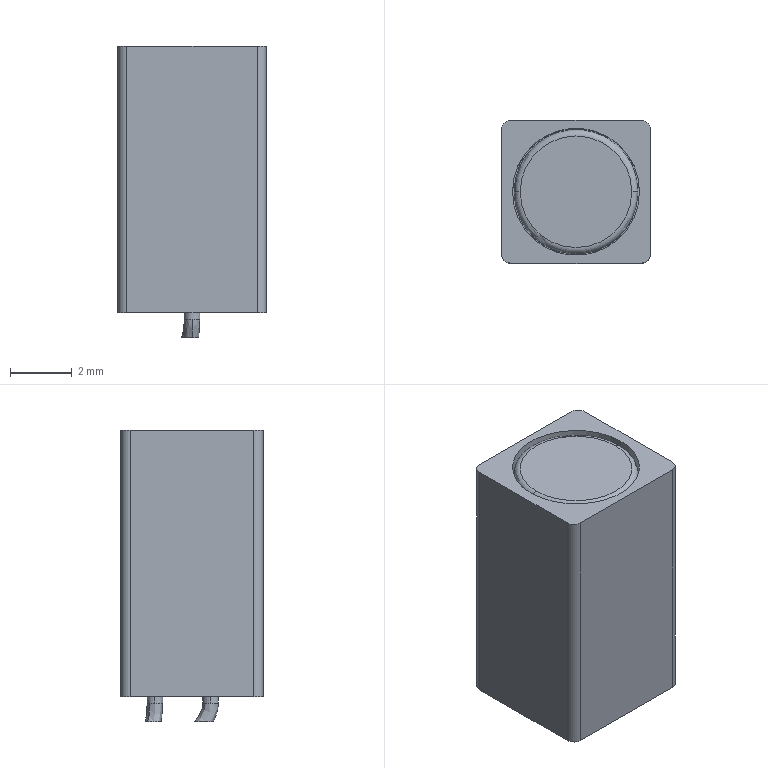Part | Creo | 1 solid | 33 faces | box 4.8 x 4.6 x 9.4 mm | volume 182.133 mm3 | cylinder 14 | plane 13 | spline 4 | torus 2 | commonest cylinder face diameters 0.5 x4 0.6 x4 0.98 x2 4 x2 4.1 x2
STEP:
#1=CARTESIAN_POINT('',(0.,0.,0.));
#2=DIRECTION('',(0.,0.,1.));
#3=DIRECTION('',(1.,0.,0.));
#4=AXIS2_PLACEMENT_3D('',#1,#2,#3);
#5=CARTESIAN_POINT('',(2.498,1.613,-0.6));
#6=VERTEX_POINT('',#5);
#7=CARTESIAN_POINT('',(2.417,2.21,-0.6));
#8=VERTEX_POINT('',#7);
#9=CARTESIAN_POINT('',(2.508,1.614,-0.6));
#10=CARTESIAN_POINT('',(2.527,1.617,-0.6));
#11=CARTESIAN_POINT('',(2.557,1.626,-0.6));
#12=CARTESIAN_POINT('',(2.585,1.64,-0.6));
#13=CARTESIAN_POINT('',(2.612,1.657,-0.6));
#14=CARTESIAN_POINT('',(2.636,1.678,-0.6));
#15=CARTESIAN_POINT('',(2.658,1.703,-0.6));
#16=CARTESIAN_POINT('',(2.676,1.73,-0.6));
#17=CARTESIAN_POINT('',(2.692,1.762,-0.6));
#18=CARTESIAN_POINT('',(2.704,1.798,-0.6));
#19=CARTESIAN_POINT('',(2.712,1.836,-0.6));
#20=CARTESIAN_POINT('',(2.715,1.877,-0.6));
#21=CARTESIAN_POINT('',(2.713,1.918,-0.6));
#22=CARTESIAN_POINT('',(2.706,1.959,-0.6));
#23=CARTESIAN_POINT('',(2.693,2.001,-0.6));
#24=CARTESIAN_POINT('',(2.675,2.043,-0.6));
#25=CARTESIAN_POINT('',(2.652,2.08,-0.6));
#26=CARTESIAN_POINT('',(2.626,2.114,-0.6));
#27=CARTESIAN_POINT('',(2.598,2.142,-0.6));
#28=CARTESIAN_POINT('',(2.568,2.166,-0.6));
#29=CARTESIAN_POINT('',(2.537,2.184,-0.6));
#30=CARTESIAN_POINT('',(2.505,2.198,-0.6));
#31=CARTESIAN_POINT('',(2.474,2.207,-0.6));
#32=CARTESIAN_POINT('',(2.444,2.211,-0.6));
#33=CARTESIAN_POINT('',(2.426,2.211,-0.6));
#34=B_SPLINE_CURVE_WITH_KNOTS('',3,(#5,#9,#10,#11,#12,#13,#14,#15,#16,#17,#18,#19,#20,#21,#22,#23,#24,#25,#26,#27,#28,#29,#30,#31,#32,#33,#7),.UNSPECIFIED.,.F.,.F.,(4,1,1,1,1,1,1,1,1,1,1,1,1,1,1,1,1,1,1,1,1,1,1,1,4),(0.,0.04167,0.08333,0.125,0.1667,0.2083,0.25,0.2917,0.3333,0.375,0.4167,0.4583,0.5,0.5417,0.5833,0.625,0.6667,0.7083,0.75,0.7917,0.8333,0.875,0.9167,0.9583,1.),.UNSPECIFIED.);
#35=EDGE_CURVE('',#6,#8,#34,.T.);
#36=ORIENTED_EDGE('',*,*,#35,.F.);
#37=CARTESIAN_POINT('',(2.526,1.451,0.));
#38=VERTEX_POINT('',#37);
#39=CARTESIAN_POINT('',(2.498,1.613,-0.6));
#40=CARTESIAN_POINT('',(2.506,1.577,-0.5309));
#41=CARTESIAN_POINT('',(2.521,1.494,-0.3468));
#42=CARTESIAN_POINT('',(2.526,1.451,-0.1342));
#43=B_SPLINE_CURVE_WITH_KNOTS('',3,(#39,#40,#41,#42,#37),.UNSPECIFIED.,.F.,.F.,(4,1,4),(0.,0.3969,1.),.UNSPECIFIED.);
#44=EDGE_CURVE('',#6,#38,#43,.T.);
#45=ORIENTED_EDGE('',*,*,#44,.T.);
#46=CARTESIAN_POINT('',(2.75,1.7,0.));
#47=VERTEX_POINT('',#46);
#48=CARTESIAN_POINT('',(2.5,1.7,0.));
#49=DIRECTION('',(0.,0.,1.));
#50=DIRECTION('',(0.1037,-0.9946,0.));
#51=AXIS2_PLACEMENT_3D('',#48,#49,#50);
#52=CIRCLE('',#51,0.25);
#53=EDGE_CURVE('',#38,#47,#52,.T.);
#54=ORIENTED_EDGE('',*,*,#53,.T.);
#55=CARTESIAN_POINT('',(2.474,1.949,0.));
#56=VERTEX_POINT('',#55);
#57=CARTESIAN_POINT('',(2.5,1.7,0.));
#58=DIRECTION('',(0.,0.,1.));
#59=DIRECTION('',(1.,0.000000353,0.));
#60=AXIS2_PLACEMENT_3D('',#57,#58,#59);
#61=CIRCLE('',#60,0.25);
#62=EDGE_CURVE('',#47,#56,#61,.T.);
#63=ORIENTED_EDGE('',*,*,#62,.T.);
#64=CARTESIAN_POINT('',(2.417,2.21,-0.6));
#65=CARTESIAN_POINT('',(2.427,2.173,-0.5544));
#66=CARTESIAN_POINT('',(2.451,2.083,-0.4299));
#67=CARTESIAN_POINT('',(2.471,1.978,-0.2252));
#68=CARTESIAN_POINT('',(2.474,1.949,-0.06818));
#69=CARTESIAN_POINT('',(2.474,1.949,0.));
#70=B_SPLINE_CURVE_WITH_KNOTS('',3,(#64,#65,#66,#67,#68,#69),.UNSPECIFIED.,.F.,.F.,(4,1,1,4),(0.,0.24,0.6382,1.),.UNSPECIFIED.);
#71=EDGE_CURVE('',#8,#56,#70,.T.);
#72=ORIENTED_EDGE('',*,*,#71,.F.);
#73=EDGE_LOOP('',(#36,#45,#54,#63,#72));
#74=FACE_OUTER_BOUND('',#73,.F.);
#75=CARTESIAN_POINT('',(2.466,1.948,0.006392));
#76=CARTESIAN_POINT('',(2.466,1.947,-0.06352));
#77=CARTESIAN_POINT('',(2.464,1.976,-0.2228));
#78=CARTESIAN_POINT('',(2.443,2.083,-0.4318));
#79=CARTESIAN_POINT('',(2.419,2.175,-0.5581));
#80=CARTESIAN_POINT('',(2.407,2.214,-0.6057));
#81=CARTESIAN_POINT('',(2.469,1.948,0.006391));
#82=CARTESIAN_POINT('',(2.469,1.947,-0.06351));
#83=CARTESIAN_POINT('',(2.466,1.976,-0.2228));
#84=CARTESIAN_POINT('',(2.446,2.083,-0.4319));
#85=CARTESIAN_POINT('',(2.421,2.176,-0.5583));
#86=CARTESIAN_POINT('',(2.41,2.214,-0.6059));
#87=CARTESIAN_POINT('',(2.536,1.956,0.006376));
#88=CARTESIAN_POINT('',(2.536,1.955,-0.06333));
#89=CARTESIAN_POINT('',(2.534,1.984,-0.2235));
#90=CARTESIAN_POINT('',(2.513,2.093,-0.4355));
#91=CARTESIAN_POINT('',(2.488,2.187,-0.5639));
#92=CARTESIAN_POINT('',(2.477,2.226,-0.6123));
#93=CARTESIAN_POINT('',(2.675,1.915,0.007061));
#94=CARTESIAN_POINT('',(2.675,1.914,-0.07018));
#95=CARTESIAN_POINT('',(2.672,1.946,-0.2451));
#96=CARTESIAN_POINT('',(2.649,2.063,-0.4733));
#97=CARTESIAN_POINT('',(2.623,2.163,-0.6099));
#98=CARTESIAN_POINT('',(2.611,2.204,-0.6613));
#99=CARTESIAN_POINT('',(2.776,1.729,0.009505));
#100=CARTESIAN_POINT('',(2.776,1.727,-0.09468));
#101=CARTESIAN_POINT('',(2.772,1.769,-0.3159));
#102=CARTESIAN_POINT('',(2.745,1.908,-0.5835));
#103=CARTESIAN_POINT('',(2.715,2.02,-0.7374));
#104=CARTESIAN_POINT('',(2.701,2.067,-0.7945));
#105=CARTESIAN_POINT('',(2.715,1.526,0.01195));
#106=CARTESIAN_POINT('',(2.715,1.524,-0.1193));
#107=CARTESIAN_POINT('',(2.71,1.576,-0.3841));
#108=CARTESIAN_POINT('',(2.68,1.732,-0.6839));
#109=CARTESIAN_POINT('',(2.647,1.854,-0.8498));
#110=CARTESIAN_POINT('',(2.633,1.903,-0.9108));
#111=CARTESIAN_POINT('',(2.588,1.457,0.01264));
#112=CARTESIAN_POINT('',(2.589,1.455,-0.1262));
#113=CARTESIAN_POINT('',(2.583,1.51,-0.4016));
#114=CARTESIAN_POINT('',(2.552,1.669,-0.7055));
#115=CARTESIAN_POINT('',(2.519,1.79,-0.8713));
#116=CARTESIAN_POINT('',(2.505,1.84,-0.9321));
#117=CARTESIAN_POINT('',(2.521,1.451,0.01263));
#118=CARTESIAN_POINT('',(2.521,1.449,-0.1261));
#119=CARTESIAN_POINT('',(2.515,1.504,-0.4002));
#120=CARTESIAN_POINT('',(2.485,1.661,-0.7008));
#121=CARTESIAN_POINT('',(2.453,1.781,-0.8644));
#122=CARTESIAN_POINT('',(2.438,1.83,-0.9243));
#123=CARTESIAN_POINT('',(2.518,1.451,0.01263));
#124=CARTESIAN_POINT('',(2.518,1.449,-0.1261));
#125=CARTESIAN_POINT('',(2.513,1.504,-0.4001));
#126=CARTESIAN_POINT('',(2.482,1.661,-0.7006));
#127=CARTESIAN_POINT('',(2.45,1.781,-0.8641));
#128=CARTESIAN_POINT('',(2.436,1.829,-0.924));
#129=B_SPLINE_SURFACE_WITH_KNOTS('',3,3,((#75,#76,#77,#78,#79,#80),(#81,#82,#83,#84,#85,#86),(#87,#88,#89,#90,#91,#92),(#93,#94,#95,#96,#97,#98),(#99,#100,#101,#102,#103,#104),(#105,#106,#107,#108,#109,#110),(#111,#112,#113,#114,#115,#116),(#117,#118,#119,#120,#121,#122),(#123,#124,#125,#126,#127,#128)),.UNSPECIFIED.,.F.,.F.,.F.,(4,1,1,1,1,1,4),(4,1,1,4),(-0.004999,0.,0.125,0.25,0.375,0.5,0.505),(-0.009526,0.304,0.6386,0.8497),.UNSPECIFIED.);
#130=ADVANCED_FACE('',(#74),#129,.T.);
#131=ORIENTED_EDGE('',*,*,#35,.T.);
#132=CARTESIAN_POINT('',(2.417,2.21,-0.6));
#133=CARTESIAN_POINT('',(2.408,2.209,-0.6));
#134=CARTESIAN_POINT('',(2.39,2.207,-0.6));
#135=CARTESIAN_POINT('',(2.363,2.199,-0.6));
#136=CARTESIAN_POINT('',(2.337,2.187,-0.6));
#137=CARTESIAN_POINT('',(2.313,2.171,-0.6));
#138=CARTESIAN_POINT('',(2.289,2.15,-0.6));
#139=CARTESIAN_POINT('',(2.268,2.126,-0.6));
#140=CARTESIAN_POINT('',(2.249,2.097,-0.6));
#141=CARTESIAN_POINT('',(2.233,2.064,-0.6));
#142=CARTESIAN_POINT('',(2.22,2.025,-0.6));
#143=CARTESIAN_POINT('',(2.211,1.982,-0.6));
#144=CARTESIAN_POINT('',(2.207,1.937,-0.6));
#145=CARTESIAN_POINT('',(2.209,1.892,-0.6));
#146=CARTESIAN_POINT('',(2.217,1.848,-0.6));
#147=CARTESIAN_POINT('',(2.229,1.805,-0.6));
#148=CARTESIAN_POINT('',(2.247,1.766,-0.6));
#149=CARTESIAN_POINT('',(2.267,1.731,-0.6));
#150=CARTESIAN_POINT('',(2.291,1.7,-0.6));
#151=CARTESIAN_POINT('',(2.317,1.674,-0.6));
#152=CARTESIAN_POINT('',(2.345,1.653,-0.6));
#153=CARTESIAN_POINT('',(2.375,1.636,-0.6));
#154=CARTESIAN_POINT('',(2.406,1.623,-0.6));
#155=CARTESIAN_POINT('',(2.438,1.615,-0.6));
#156=CARTESIAN_POINT('',(2.469,1.612,-0.6));
#157=CARTESIAN_POINT('',(2.489,1.612,-0.6));
#158=CARTESIAN_POINT('',(2.498,1.613,-0.6));
#159=B_SPLINE_CURVE_WITH_KNOTS('',3,(#132,#133,#134,#135,#136,#137,#138,#139,#140,#141,#142,#143,#144,#145,#146,#147,#148,#149,#150,#151,#152,#153,#154,#155,#156,#157,#158),.UNSPECIFIED.,.F.,.F.,(4,1,1,1,1,1,1,1,1,1,1,1,1,1,1,1,1,1,1,1,1,1,1,1,4),(0.,0.04167,0.08333,0.125,0.1667,0.2083,0.25,0.2917,0.3333,0.375,0.4167,0.4583,0.5,0.5417,0.5833,0.625,0.6667,0.7083,0.75,0.7917,0.8333,0.875,0.9167,0.9583,1.),.UNSPECIFIED.);
#160=EDGE_CURVE('',#8,#6,#159,.T.);
#161=ORIENTED_EDGE('',*,*,#160,.T.);
#162=EDGE_LOOP('',(#131,#161));
#163=FACE_OUTER_BOUND('',#162,.F.);
#164=CARTESIAN_POINT('',(0.1,4.6,-0.6));
#165=DIRECTION('',(0.,0.,1.));
#166=DIRECTION('',(1.,0.,0.));
#167=AXIS2_PLACEMENT_3D('',#164,#165,#166);
#168=PLANE('',#167);
#169=ADVANCED_FACE('',(#163),#168,.F.);
#170=ORIENTED_EDGE('',*,*,#160,.F.);
#171=ORIENTED_EDGE('',*,*,#71,.T.);
#172=CARTESIAN_POINT('',(2.25,1.7,0.));
#173=VERTEX_POINT('',#172);
#174=CARTESIAN_POINT('',(2.5,1.7,0.));
#175=DIRECTION('',(0.,0.,1.));
#176=DIRECTION('',(-0.1037,0.9946,0.));
#177=AXIS2_PLACEMENT_3D('',#174,#175,#176);
#178=CIRCLE('',#177,0.25);
#179=EDGE_CURVE('',#56,#173,#178,.T.);
#180=ORIENTED_EDGE('',*,*,#179,.T.);
#181=CARTESIAN_POINT('',(2.5,1.7,0.));
#182=DIRECTION('',(0.,0.,1.));
#183=DIRECTION('',(-1.,0.,0.));
#184=AXIS2_PLACEMENT_3D('',#181,#182,#183);
#185=CIRCLE('',#184,0.25);
#186=EDGE_CURVE('',#173,#38,#185,.T.);
#187=ORIENTED_EDGE('',*,*,#186,.T.);
#188=ORIENTED_EDGE('',*,*,#44,.F.);
#189=EDGE_LOOP('',(#170,#171,#180,#187,#188));
#190=FACE_OUTER_BOUND('',#189,.F.);
#191=CARTESIAN_POINT('',(2.534,1.452,0.01264));
#192=CARTESIAN_POINT('',(2.534,1.451,-0.1261));
#193=CARTESIAN_POINT('',(2.528,1.505,-0.4003));
#194=CARTESIAN_POINT('',(2.497,1.664,-0.7026));
#195=CARTESIAN_POINT('',(2.465,1.785,-0.8674));
#196=CARTESIAN_POINT('',(2.45,1.834,-0.9282));
#197=CARTESIAN_POINT('',(2.531,1.452,0.01264));
#198=CARTESIAN_POINT('',(2.531,1.45,-0.1261));
#199=CARTESIAN_POINT('',(2.526,1.505,-0.4003));
#200=CARTESIAN_POINT('',(2.495,1.663,-0.7025));
#201=CARTESIAN_POINT('',(2.462,1.784,-0.8672));
#202=CARTESIAN_POINT('',(2.448,1.833,-0.928));
#203=CARTESIAN_POINT('',(2.464,1.444,0.01265));
#204=CARTESIAN_POINT('',(2.464,1.442,-0.1263));
#205=CARTESIAN_POINT('',(2.458,1.497,-0.3997));
#206=CARTESIAN_POINT('',(2.428,1.654,-0.6989));
#207=CARTESIAN_POINT('',(2.396,1.773,-0.8616));
#208=CARTESIAN_POINT('',(2.381,1.822,-0.9216));
#209=CARTESIAN_POINT('',(2.325,1.485,0.01197));
#210=CARTESIAN_POINT('',(2.326,1.483,-0.1194));
#211=CARTESIAN_POINT('',(2.32,1.535,-0.3781));
#212=CARTESIAN_POINT('',(2.291,1.683,-0.6611));
#213=CARTESIAN_POINT('',(2.261,1.797,-0.8154));
#214=CARTESIAN_POINT('',(2.247,1.843,-0.8724));
#215=CARTESIAN_POINT('',(2.224,1.671,0.009523));
#216=CARTESIAN_POINT('',(2.225,1.67,-0.09494));
#217=CARTESIAN_POINT('',(2.22,1.712,-0.3073));
#218=CARTESIAN_POINT('',(2.196,1.838,-0.5507));
#219=CARTESIAN_POINT('',(2.169,1.939,-0.6878));
#220=CARTESIAN_POINT('',(2.157,1.981,-0.739));
#221=CARTESIAN_POINT('',(2.285,1.875,0.007075));
#222=CARTESIAN_POINT('',(2.285,1.874,-0.07036));
#223=CARTESIAN_POINT('',(2.282,1.905,-0.2391));
#224=CARTESIAN_POINT('',(2.261,2.014,-0.4501));
#225=CARTESIAN_POINT('',(2.237,2.106,-0.5752));
#226=CARTESIAN_POINT('',(2.225,2.144,-0.6225));
#227=CARTESIAN_POINT('',(2.412,1.943,0.006383));
#228=CARTESIAN_POINT('',(2.412,1.942,-0.06339));
#229=CARTESIAN_POINT('',(2.409,1.971,-0.2216));
#230=CARTESIAN_POINT('',(2.388,2.077,-0.4286));
#231=CARTESIAN_POINT('',(2.364,2.169,-0.5537));
#232=CARTESIAN_POINT('',(2.353,2.208,-0.6012));
#233=CARTESIAN_POINT('',(2.479,1.949,0.006395));
#234=CARTESIAN_POINT('',(2.479,1.948,-0.0635));
#235=CARTESIAN_POINT('',(2.477,1.977,-0.223));
#236=CARTESIAN_POINT('',(2.456,2.085,-0.4333));
#237=CARTESIAN_POINT('',(2.431,2.178,-0.5607));
#238=CARTESIAN_POINT('',(2.42,2.218,-0.609));
#239=CARTESIAN_POINT('',(2.482,1.949,0.006396));
#240=CARTESIAN_POINT('',(2.482,1.948,-0.06351));
#241=CARTESIAN_POINT('',(2.479,1.977,-0.2231));
#242=CARTESIAN_POINT('',(2.458,2.085,-0.4335));
#243=CARTESIAN_POINT('',(2.434,2.179,-0.561));
#244=CARTESIAN_POINT('',(2.422,2.218,-0.6094));
#245=B_SPLINE_SURFACE_WITH_KNOTS('',3,3,((#191,#192,#193,#194,#195,#196),(#197,#198,#199,#200,#201,#202),(#203,#204,#205,#206,#207,#208),(#209,#210,#211,#212,#213,#214),(#215,#216,#217,#218,#219,#220),(#221,#222,#223,#224,#225,#226),(#227,#228,#229,#230,#231,#232),(#233,#234,#235,#236,#237,#238),(#239,#240,#241,#242,#243,#244)),.UNSPECIFIED.,.F.,.F.,.F.,(4,1,1,1,1,1,4),(4,1,1,4),(0.495,0.5,0.625,0.75,0.875,1.,1.005),(-0.009533,0.304,0.6386,0.8527),.UNSPECIFIED.);
#246=ADVANCED_FACE('',(#190),#245,.T.);
#247=CARTESIAN_POINT('',(2.75,1.7,0.7));
#248=VERTEX_POINT('',#247);
#249=CARTESIAN_POINT('',(2.75,1.7,0.7));
#250=DIRECTION('',(-0.00002824,0.000000111,-1.));
#251=VECTOR('',#250,0.7);
#252=LINE('',#249,#251);
#253=EDGE_CURVE('',#248,#47,#252,.T.);
#254=ORIENTED_EDGE('',*,*,#253,.F.);
#255=CARTESIAN_POINT('',(2.25,1.7,0.7));
#256=VERTEX_POINT('',#255);
#257=CARTESIAN_POINT('',(2.5,1.7,0.7));
#258=DIRECTION('',(0.,0.,-1.));
#259=DIRECTION('',(-1.,-0.000000032,0.));
#260=AXIS2_PLACEMENT_3D('',#257,#258,#259);
#261=CIRCLE('',#260,0.25);
#262=EDGE_CURVE('',#256,#248,#261,.T.);
#263=ORIENTED_EDGE('',*,*,#262,.F.);
#264=CARTESIAN_POINT('',(2.25,1.7,0.));
#265=DIRECTION('',(-0.00002824,0.000000107,1.));
#266=VECTOR('',#265,0.7);
#267=LINE('',#264,#266);
#268=EDGE_CURVE('',#173,#256,#267,.T.);
#269=ORIENTED_EDGE('',*,*,#268,.F.);
#270=ORIENTED_EDGE('',*,*,#179,.F.);
#271=ORIENTED_EDGE('',*,*,#62,.F.);
#272=EDGE_LOOP('',(#254,#263,#269,#270,#271));
#273=FACE_OUTER_BOUND('',#272,.F.);
#274=CARTESIAN_POINT('',(2.5,1.7,0.2));
#275=DIRECTION('',(0.,0.,-1.));
#276=DIRECTION('',(-1.,0.,0.));
#277=AXIS2_PLACEMENT_3D('',#274,#275,#276);
#278=CYLINDRICAL_SURFACE('',#277,0.25);
#279=ADVANCED_FACE('',(#273),#278,.T.);
#280=ORIENTED_EDGE('',*,*,#268,.T.);
#281=CARTESIAN_POINT('',(2.5,1.7,0.7));
#282=DIRECTION('',(0.,0.,-1.));
#283=DIRECTION('',(1.,0.000000127,0.));
#284=AXIS2_PLACEMENT_3D('',#281,#282,#283);
#285=CIRCLE('',#284,0.25);
#286=EDGE_CURVE('',#248,#256,#285,.T.);
#287=ORIENTED_EDGE('',*,*,#286,.F.);
#288=ORIENTED_EDGE('',*,*,#253,.T.);
#289=ORIENTED_EDGE('',*,*,#53,.F.);
#290=ORIENTED_EDGE('',*,*,#186,.F.);
#291=EDGE_LOOP('',(#280,#287,#288,#289,#290));
#292=FACE_OUTER_BOUND('',#291,.F.);
#293=CARTESIAN_POINT('',(2.5,1.7,0.2));
#294=DIRECTION('',(0.,0.,-1.));
#295=DIRECTION('',(-1.,0.,0.));
#296=AXIS2_PLACEMENT_3D('',#293,#294,#295);
#297=CYLINDRICAL_SURFACE('',#296,0.25);
#298=ADVANCED_FACE('',(#292),#297,.T.);
#299=CARTESIAN_POINT('',(2.99,3.78,0.7));
#300=VERTEX_POINT('',#299);
#301=CARTESIAN_POINT('',(2.01,3.78,0.7));
#302=VERTEX_POINT('',#301);
#303=CARTESIAN_POINT('',(2.5,3.78,0.7));
#304=DIRECTION('',(0.,0.,1.));
#305=DIRECTION('',(1.,0.,0.));
#306=AXIS2_PLACEMENT_3D('',#303,#304,#305);
#307=CIRCLE('',#306,0.49);
#308=EDGE_CURVE('',#300,#302,#307,.T.);
#309=ORIENTED_EDGE('',*,*,#308,.T.);
#310=CARTESIAN_POINT('',(2.01,0.9,0.7));
#311=VERTEX_POINT('',#310);
#312=CARTESIAN_POINT('',(2.01,3.78,0.7));
#313=DIRECTION('',(0.,-1.,0.));
#314=VECTOR('',#313,2.88);
#315=LINE('',#312,#314);
#316=EDGE_CURVE('',#302,#311,#315,.T.);
#317=ORIENTED_EDGE('',*,*,#316,.T.);
#318=CARTESIAN_POINT('',(2.99,0.9,0.7));
#319=VERTEX_POINT('',#318);
#320=CARTESIAN_POINT('',(2.5,0.9,0.7));
#321=DIRECTION('',(0.,0.,1.));
#322=DIRECTION('',(-1.,0.,0.));
#323=AXIS2_PLACEMENT_3D('',#320,#321,#322);
#324=CIRCLE('',#323,0.49);
#325=EDGE_CURVE('',#311,#319,#324,.T.);
#326=ORIENTED_EDGE('',*,*,#325,.T.);
#327=CARTESIAN_POINT('',(2.99,0.9,0.7));
#328=DIRECTION('',(0.,1.,0.));
#329=VECTOR('',#328,2.88);
#330=LINE('',#327,#329);
#331=EDGE_CURVE('',#319,#300,#330,.T.);
#332=ORIENTED_EDGE('',*,*,#331,.T.);
#333=EDGE_LOOP('',(#309,#317,#326,#332));
#334=FACE_OUTER_BOUND('',#333,.F.);
#335=CARTESIAN_POINT('',(2.75,3.5,0.7));
#336=VERTEX_POINT('',#335);
#337=CARTESIAN_POINT('',(2.25,3.5,0.7));
#338=VERTEX_POINT('',#337);
#339=CARTESIAN_POINT('',(2.5,3.5,0.7));
#340=DIRECTION('',(0.,0.,-1.));
#341=DIRECTION('',(1.,0.,0.));
#342=AXIS2_PLACEMENT_3D('',#339,#340,#341);
#343=CIRCLE('',#342,0.25);
#344=EDGE_CURVE('',#336,#338,#343,.T.);
#345=ORIENTED_EDGE('',*,*,#344,.T.);
#346=CARTESIAN_POINT('',(2.5,3.5,0.7));
#347=DIRECTION('',(0.,0.,-1.));
#348=DIRECTION('',(-1.,0.,0.));
#349=AXIS2_PLACEMENT_3D('',#346,#347,#348);
#350=CIRCLE('',#349,0.25);
#351=EDGE_CURVE('',#338,#336,#350,.T.);
#352=ORIENTED_EDGE('',*,*,#351,.T.);
#353=EDGE_LOOP('',(#345,#352));
#354=FACE_BOUND('',#353,.F.);
#355=ORIENTED_EDGE('',*,*,#286,.T.);
#356=ORIENTED_EDGE('',*,*,#262,.T.);
#357=EDGE_LOOP('',(#355,#356));
#358=FACE_BOUND('',#357,.F.);
#359=CARTESIAN_POINT('',(0.,0.,0.7));
#360=DIRECTION('',(0.,0.,-1.));
#361=DIRECTION('',(-1.,0.,0.));
#362=AXIS2_PLACEMENT_3D('',#359,#360,#361);
#363=PLANE('',#362);
#364=ADVANCED_FACE('',(#334,#354,#358),#363,.T.);
#365=CARTESIAN_POINT('',(2.01,3.78,0.2));
#366=VERTEX_POINT('',#365);
#367=CARTESIAN_POINT('',(2.99,3.78,0.2));
#368=VERTEX_POINT('',#367);
#369=CARTESIAN_POINT('',(2.5,3.78,0.2));
#370=DIRECTION('',(0.,0.,-1.));
#371=DIRECTION('',(-1.,0.,0.));
#372=AXIS2_PLACEMENT_3D('',#369,#370,#371);
#373=CIRCLE('',#372,0.49);
#374=EDGE_CURVE('',#366,#368,#373,.T.);
#375=ORIENTED_EDGE('',*,*,#374,.F.);
#376=CARTESIAN_POINT('',(2.01,3.78,0.2));
#377=DIRECTION('',(0.,0.,1.));
#378=VECTOR('',#377,0.5);
#379=LINE('',#376,#378);
#380=EDGE_CURVE('',#366,#302,#379,.T.);
#381=ORIENTED_EDGE('',*,*,#380,.T.);
#382=ORIENTED_EDGE('',*,*,#308,.F.);
#383=CARTESIAN_POINT('',(2.99,3.78,0.7));
#384=DIRECTION('',(0.,0.,-1.));
#385=VECTOR('',#384,0.5);
#386=LINE('',#383,#385);
#387=EDGE_CURVE('',#300,#368,#386,.T.);
#388=ORIENTED_EDGE('',*,*,#387,.T.);
#389=EDGE_LOOP('',(#375,#381,#382,#388));
#390=FACE_OUTER_BOUND('',#389,.F.);
#391=CARTESIAN_POINT('',(2.5,3.78,0.2));
#392=DIRECTION('',(0.,0.,-1.));
#393=DIRECTION('',(-1.,0.,0.));
#394=AXIS2_PLACEMENT_3D('',#391,#392,#393);
#395=CYLINDRICAL_SURFACE('',#394,0.49);
#396=ADVANCED_FACE('',(#390),#395,.F.);
#397=CARTESIAN_POINT('',(4.9,4.3,0.2));
#398=VERTEX_POINT('',#397);
#399=CARTESIAN_POINT('',(4.6,4.6,0.2));
#400=VERTEX_POINT('',#399);
#401=CARTESIAN_POINT('',(4.6,4.3,0.2));
#402=DIRECTION('',(0.,0.,1.));
#403=DIRECTION('',(1.,-0.000000002,0.));
#404=AXIS2_PLACEMENT_3D('',#401,#402,#403);
#405=CIRCLE('',#404,0.3);
#406=EDGE_CURVE('',#398,#400,#405,.T.);
#407=ORIENTED_EDGE('',*,*,#406,.T.);
#408=CARTESIAN_POINT('',(0.4,4.6,0.2));
#409=VERTEX_POINT('',#408);
#410=CARTESIAN_POINT('',(4.6,4.6,0.2));
#411=DIRECTION('',(-1.,0.,0.));
#412=VECTOR('',#411,4.2);
#413=LINE('',#410,#412);
#414=EDGE_CURVE('',#400,#409,#413,.T.);
#415=ORIENTED_EDGE('',*,*,#414,.T.);
#416=CARTESIAN_POINT('',(0.1,4.3,0.2));
#417=VERTEX_POINT('',#416);
#418=CARTESIAN_POINT('',(0.4,4.3,0.2));
#419=DIRECTION('',(0.,0.,1.));
#420=DIRECTION('',(0.,1.,0.));
#421=AXIS2_PLACEMENT_3D('',#418,#419,#420);
#422=CIRCLE('',#421,0.3);
#423=EDGE_CURVE('',#409,#417,#422,.T.);
#424=ORIENTED_EDGE('',*,*,#423,.T.);
#425=CARTESIAN_POINT('',(0.1,0.3,0.2));
#426=VERTEX_POINT('',#425);
#427=CARTESIAN_POINT('',(0.1,4.3,0.2));
#428=DIRECTION('',(0.,-1.,0.));
#429=VECTOR('',#428,4.);
#430=LINE('',#427,#429);
#431=EDGE_CURVE('',#417,#426,#430,.T.);
#432=ORIENTED_EDGE('',*,*,#431,.T.);
#433=CARTESIAN_POINT('',(0.4,0.,0.2));
#434=VERTEX_POINT('',#433);
#435=CARTESIAN_POINT('',(0.4,0.3,0.2));
#436=DIRECTION('',(0.,0.,1.));
#437=DIRECTION('',(-1.,0.000000002,0.));
#438=AXIS2_PLACEMENT_3D('',#435,#436,#437);
#439=CIRCLE('',#438,0.3);
#440=EDGE_CURVE('',#426,#434,#439,.T.);
#441=ORIENTED_EDGE('',*,*,#440,.T.);
#442=CARTESIAN_POINT('',(4.6,0.,0.2));
#443=VERTEX_POINT('',#442);
#444=CARTESIAN_POINT('',(0.4,0.,0.2));
#445=DIRECTION('',(1.,0.,0.));
#446=VECTOR('',#445,4.2);
#447=LINE('',#444,#446);
#448=EDGE_CURVE('',#434,#443,#447,.T.);
#449=ORIENTED_EDGE('',*,*,#448,.T.);
#450=CARTESIAN_POINT('',(4.9,0.3,0.2));
#451=VERTEX_POINT('',#450);
#452=CARTESIAN_POINT('',(4.6,0.3,0.2));
#453=DIRECTION('',(0.,0.,1.));
#454=DIRECTION('',(0.,-1.,0.));
#455=AXIS2_PLACEMENT_3D('',#452,#453,#454);
#456=CIRCLE('',#455,0.3);
#457=EDGE_CURVE('',#443,#451,#456,.T.);
#458=ORIENTED_EDGE('',*,*,#457,.T.);
#459=CARTESIAN_POINT('',(4.9,0.3,0.2));
#460=DIRECTION('',(0.,1.,0.));
#461=VECTOR('',#460,4.);
#462=LINE('',#459,#461);
#463=EDGE_CURVE('',#451,#398,#462,.T.);
#464=ORIENTED_EDGE('',*,*,#463,.T.);
#465=EDGE_LOOP('',(#407,#415,#424,#432,#441,#449,#458,#464));
#466=FACE_OUTER_BOUND('',#465,.F.);
#467=ORIENTED_EDGE('',*,*,#374,.T.);
#468=CARTESIAN_POINT('',(2.99,0.9,0.2));
#469=VERTEX_POINT('',#468);
#470=CARTESIAN_POINT('',(2.99,0.9,0.2));
#471=DIRECTION('',(0.,1.,0.));
#472=VECTOR('',#471,2.88);
#473=LINE('',#470,#472);
#474=EDGE_CURVE('',#469,#368,#473,.T.);
#475=ORIENTED_EDGE('',*,*,#474,.F.);
#476=CARTESIAN_POINT('',(2.01,0.9,0.2));
#477=VERTEX_POINT('',#476);
#478=CARTESIAN_POINT('',(2.5,0.9,0.2));
#479=DIRECTION('',(0.,0.,-1.));
#480=DIRECTION('',(1.,0.,0.));
#481=AXIS2_PLACEMENT_3D('',#478,#479,#480);
#482=CIRCLE('',#481,0.49);
#483=EDGE_CURVE('',#469,#477,#482,.T.);
#484=ORIENTED_EDGE('',*,*,#483,.T.);
#485=CARTESIAN_POINT('',(2.01,3.78,0.2));
#486=DIRECTION('',(0.,-1.,0.));
#487=VECTOR('',#486,2.88);
#488=LINE('',#485,#487);
#489=EDGE_CURVE('',#366,#477,#488,.T.);
#490=ORIENTED_EDGE('',*,*,#489,.F.);
#491=EDGE_LOOP('',(#467,#475,#484,#490));
#492=FACE_BOUND('',#491,.F.);
#493=CARTESIAN_POINT('',(0.,0.,0.2));
#494=DIRECTION('',(0.,0.,-1.));
#495=DIRECTION('',(-1.,0.,0.));
#496=AXIS2_PLACEMENT_3D('',#493,#494,#495);
#497=PLANE('',#496);
#498=ADVANCED_FACE('',(#466,#492),#497,.T.);
#499=CARTESIAN_POINT('',(4.9,4.3,8.8));
#500=VERTEX_POINT('',#499);
#501=CARTESIAN_POINT('',(4.9,4.3,0.2));
#502=DIRECTION('',(0.,0.,1.));
#503=VECTOR('',#502,8.6);
#504=LINE('',#501,#503);
#505=EDGE_CURVE('',#398,#500,#504,.T.);
#506=ORIENTED_EDGE('',*,*,#505,.T.);
#507=CARTESIAN_POINT('',(4.6,4.6,8.8));
#508=VERTEX_POINT('',#507);
#509=CARTESIAN_POINT('',(4.6,4.3,8.8));
#510=DIRECTION('',(0.,0.,-1.));
#511=DIRECTION('',(0.,1.,0.));
#512=AXIS2_PLACEMENT_3D('',#509,#510,#511);
#513=CIRCLE('',#512,0.3);
#514=EDGE_CURVE('',#508,#500,#513,.T.);
#515=ORIENTED_EDGE('',*,*,#514,.F.);
#516=CARTESIAN_POINT('',(4.6,4.6,8.8));
#517=DIRECTION('',(0.,0.,-1.));
#518=VECTOR('',#517,8.6);
#519=LINE('',#516,#518);
#520=EDGE_CURVE('',#508,#400,#519,.T.);
#521=ORIENTED_EDGE('',*,*,#520,.T.);
#522=ORIENTED_EDGE('',*,*,#406,.F.);
#523=EDGE_LOOP('',(#506,#515,#521,#522));
#524=FACE_OUTER_BOUND('',#523,.F.);
#525=CARTESIAN_POINT('',(4.6,4.3,37.611));
#526=DIRECTION('',(0.,0.,-1.));
#527=DIRECTION('',(0.,1.,0.));
#528=AXIS2_PLACEMENT_3D('',#525,#526,#527);
#529=CYLINDRICAL_SURFACE('',#528,0.3);
#530=ADVANCED_FACE('',(#524),#529,.T.);
#531=CARTESIAN_POINT('',(4.9,0.3,8.8));
#532=VERTEX_POINT('',#531);
#533=CARTESIAN_POINT('',(4.9,0.3,8.8));
#534=DIRECTION('',(0.,0.,-1.));
#535=VECTOR('',#534,8.6);
#536=LINE('',#533,#535);
#537=EDGE_CURVE('',#532,#451,#536,.T.);
#538=ORIENTED_EDGE('',*,*,#537,.F.);
#539=CARTESIAN_POINT('',(4.9,0.3,8.8));
#540=DIRECTION('',(0.,1.,0.));
#541=VECTOR('',#540,4.);
#542=LINE('',#539,#541);
#543=EDGE_CURVE('',#532,#500,#542,.T.);
#544=ORIENTED_EDGE('',*,*,#543,.T.);
#545=ORIENTED_EDGE('',*,*,#505,.F.);
#546=ORIENTED_EDGE('',*,*,#463,.F.);
#547=EDGE_LOOP('',(#538,#544,#545,#546));
#548=FACE_OUTER_BOUND('',#547,.F.);
#549=CARTESIAN_POINT('',(4.9,0.,8.8));
#550=DIRECTION('',(-1.,0.,0.));
#551=DIRECTION('',(0.,0.,-1.));
#552=AXIS2_PLACEMENT_3D('',#549,#550,#551);
#553=PLANE('',#552);
#554=ADVANCED_FACE('',(#548),#553,.F.);
#555=CARTESIAN_POINT('',(4.6,0.,8.8));
#556=VERTEX_POINT('',#555);
#557=CARTESIAN_POINT('',(4.6,0.,0.2));
#558=DIRECTION('',(0.,0.,1.));
#559=VECTOR('',#558,8.6);
#560=LINE('',#557,#559);
#561=EDGE_CURVE('',#443,#556,#560,.T.);
#562=ORIENTED_EDGE('',*,*,#561,.T.);
#563=CARTESIAN_POINT('',(4.6,0.3,8.8));
#564=DIRECTION('',(0.,0.,-1.));
#565=DIRECTION('',(1.,0.,0.));
#566=AXIS2_PLACEMENT_3D('',#563,#564,#565);
#567=CIRCLE('',#566,0.3);
#568=EDGE_CURVE('',#532,#556,#567,.T.);
#569=ORIENTED_EDGE('',*,*,#568,.F.);
#570=ORIENTED_EDGE('',*,*,#537,.T.);
#571=ORIENTED_EDGE('',*,*,#457,.F.);
#572=EDGE_LOOP('',(#562,#569,#570,#571));
#573=FACE_OUTER_BOUND('',#572,.F.);
#574=CARTESIAN_POINT('',(4.6,0.3,-33.811));
#575=DIRECTION('',(0.,0.,1.));
#576=DIRECTION('',(0.,-1.,0.));
#577=AXIS2_PLACEMENT_3D('',#574,#575,#576);
#578=CYLINDRICAL_SURFACE('',#577,0.3);
#579=ADVANCED_FACE('',(#573),#578,.T.);
#580=CARTESIAN_POINT('',(0.4,0.,8.8));
#581=VERTEX_POINT('',#580);
#582=CARTESIAN_POINT('',(0.4,0.,8.8));
#583=DIRECTION('',(0.,0.,-1.));
#584=VECTOR('',#583,8.6);
#585=LINE('',#582,#584);
#586=EDGE_CURVE('',#581,#434,#585,.T.);
#587=ORIENTED_EDGE('',*,*,#586,.F.);
#588=CARTESIAN_POINT('',(0.4,0.,8.8));
#589=DIRECTION('',(1.,0.,0.));
#590=VECTOR('',#589,4.2);
#591=LINE('',#588,#590);
#592=EDGE_CURVE('',#581,#556,#591,.T.);
#593=ORIENTED_EDGE('',*,*,#592,.T.);
#594=ORIENTED_EDGE('',*,*,#561,.F.);
#595=ORIENTED_EDGE('',*,*,#448,.F.);
#596=EDGE_LOOP('',(#587,#593,#594,#595));
#597=FACE_OUTER_BOUND('',#596,.F.);
#598=CARTESIAN_POINT('',(0.,0.,0.));
#599=DIRECTION('',(0.,-1.,0.));
#600=DIRECTION('',(1.,0.,0.));
#601=AXIS2_PLACEMENT_3D('',#598,#599,#600);
#602=PLANE('',#601);
#603=ADVANCED_FACE('',(#597),#602,.T.);
#604=ORIENTED_EDGE('',*,*,#586,.T.);
#605=ORIENTED_EDGE('',*,*,#440,.F.);
#606=CARTESIAN_POINT('',(0.1,0.3,8.8));
#607=VERTEX_POINT('',#606);
#608=CARTESIAN_POINT('',(0.1,0.3,0.2));
#609=DIRECTION('',(0.,0.,1.));
#610=VECTOR('',#609,8.6);
#611=LINE('',#608,#610);
#612=EDGE_CURVE('',#426,#607,#611,.T.);
#613=ORIENTED_EDGE('',*,*,#612,.T.);
#614=CARTESIAN_POINT('',(0.4,0.3,8.8));
#615=DIRECTION('',(0.,0.,-1.));
#616=DIRECTION('',(0.,-1.,0.));
#617=AXIS2_PLACEMENT_3D('',#614,#615,#616);
#618=CIRCLE('',#617,0.3);
#619=EDGE_CURVE('',#581,#607,#618,.T.);
#620=ORIENTED_EDGE('',*,*,#619,.F.);
#621=EDGE_LOOP('',(#604,#605,#613,#620));
#622=FACE_OUTER_BOUND('',#621,.F.);
#623=CARTESIAN_POINT('',(0.4,0.3,37.611));
#624=DIRECTION('',(0.,0.,-1.));
#625=DIRECTION('',(0.,-1.,0.));
#626=AXIS2_PLACEMENT_3D('',#623,#624,#625);
#627=CYLINDRICAL_SURFACE('',#626,0.3);
#628=ADVANCED_FACE('',(#622),#627,.T.);
#629=ORIENTED_EDGE('',*,*,#612,.F.);
#630=ORIENTED_EDGE('',*,*,#431,.F.);
#631=CARTESIAN_POINT('',(0.1,4.3,8.8));
#632=VERTEX_POINT('',#631);
#633=CARTESIAN_POINT('',(0.1,4.3,8.8));
#634=DIRECTION('',(0.,0.,-1.));
#635=VECTOR('',#634,8.6);
#636=LINE('',#633,#635);
#637=EDGE_CURVE('',#632,#417,#636,.T.);
#638=ORIENTED_EDGE('',*,*,#637,.F.);
#639=CARTESIAN_POINT('',(0.1,4.3,8.8));
#640=DIRECTION('',(0.,-1.,0.));
#641=VECTOR('',#640,4.);
#642=LINE('',#639,#641);
#643=EDGE_CURVE('',#632,#607,#642,.T.);
#644=ORIENTED_EDGE('',*,*,#643,.T.);
#645=EDGE_LOOP('',(#629,#630,#638,#644));
#646=FACE_OUTER_BOUND('',#645,.F.);
#647=CARTESIAN_POINT('',(0.1,0.,0.));
#648=DIRECTION('',(1.,0.,0.));
#649=DIRECTION('',(0.,0.,1.));
#650=AXIS2_PLACEMENT_3D('',#647,#648,#649);
#651=PLANE('',#650);
#652=ADVANCED_FACE('',(#646),#651,.F.);
#653=CARTESIAN_POINT('',(0.4,4.6,8.8));
#654=VERTEX_POINT('',#653);
#655=CARTESIAN_POINT('',(0.4,4.6,0.2));
#656=DIRECTION('',(0.,0.,1.));
#657=VECTOR('',#656,8.6);
#658=LINE('',#655,#657);
#659=EDGE_CURVE('',#409,#654,#658,.T.);
#660=ORIENTED_EDGE('',*,*,#659,.T.);
#661=CARTESIAN_POINT('',(0.4,4.3,8.8));
#662=DIRECTION('',(0.,0.,-1.));
#663=DIRECTION('',(-1.,0.,0.));
#664=AXIS2_PLACEMENT_3D('',#661,#662,#663);
#665=CIRCLE('',#664,0.3);
#666=EDGE_CURVE('',#632,#654,#665,.T.);
#667=ORIENTED_EDGE('',*,*,#666,.F.);
#668=ORIENTED_EDGE('',*,*,#637,.T.);
#669=ORIENTED_EDGE('',*,*,#423,.F.);
#670=EDGE_LOOP('',(#660,#667,#668,#669));
#671=FACE_OUTER_BOUND('',#670,.F.);
#672=CARTESIAN_POINT('',(0.4,4.3,-33.811));
#673=DIRECTION('',(0.,0.,1.));
#674=DIRECTION('',(0.,1.,0.));
#675=AXIS2_PLACEMENT_3D('',#672,#673,#674);
#676=CYLINDRICAL_SURFACE('',#675,0.3);
#677=ADVANCED_FACE('',(#671),#676,.T.);
#678=ORIENTED_EDGE('',*,*,#520,.F.);
#679=CARTESIAN_POINT('',(4.6,4.6,8.8));
#680=DIRECTION('',(-1.,0.,0.));
#681=VECTOR('',#680,4.2);
#682=LINE('',#679,#681);
#683=EDGE_CURVE('',#508,#654,#682,.T.);
#684=ORIENTED_EDGE('',*,*,#683,.T.);
#685=ORIENTED_EDGE('',*,*,#659,.F.);
#686=ORIENTED_EDGE('',*,*,#414,.F.);
#687=EDGE_LOOP('',(#678,#684,#685,#686));
#688=FACE_OUTER_BOUND('',#687,.F.);
#689=CARTESIAN_POINT('',(0.,4.6,0.));
#690=DIRECTION('',(0.,-1.,0.));
#691=DIRECTION('',(1.,0.,0.));
#692=AXIS2_PLACEMENT_3D('',#689,#690,#691);
#693=PLANE('',#692);
#694=ADVANCED_FACE('',(#688),#693,.F.);
#695=ORIENTED_EDGE('',*,*,#514,.T.);
#696=ORIENTED_EDGE('',*,*,#543,.F.);
#697=ORIENTED_EDGE('',*,*,#568,.T.);
#698=ORIENTED_EDGE('',*,*,#592,.F.);
#699=ORIENTED_EDGE('',*,*,#619,.T.);
#700=ORIENTED_EDGE('',*,*,#643,.F.);
#701=ORIENTED_EDGE('',*,*,#666,.T.);
#702=ORIENTED_EDGE('',*,*,#683,.F.);
#703=EDGE_LOOP('',(#695,#696,#697,#698,#699,#700,#701,#702));
#704=FACE_OUTER_BOUND('',#703,.F.);
#705=CARTESIAN_POINT('',(4.55,2.3,8.8));
#706=VERTEX_POINT('',#705);
#707=CARTESIAN_POINT('',(0.45,2.3,8.8));
#708=VERTEX_POINT('',#707);
#709=CARTESIAN_POINT('',(2.5,2.3,8.8));
#710=DIRECTION('',(0.,0.,1.));
#711=DIRECTION('',(1.,0.,0.));
#712=AXIS2_PLACEMENT_3D('',#709,#710,#711);
#713=CIRCLE('',#712,2.05);
#714=EDGE_CURVE('',#706,#708,#713,.T.);
#715=ORIENTED_EDGE('',*,*,#714,.T.);
#716=CARTESIAN_POINT('',(2.5,2.3,8.8));
#717=DIRECTION('',(0.,0.,1.));
#718=DIRECTION('',(-1.,0.,0.));
#719=AXIS2_PLACEMENT_3D('',#716,#717,#718);
#720=CIRCLE('',#719,2.05);
#721=EDGE_CURVE('',#708,#706,#720,.T.);
#722=ORIENTED_EDGE('',*,*,#721,.T.);
#723=EDGE_LOOP('',(#715,#722));
#724=FACE_BOUND('',#723,.F.);
#725=CARTESIAN_POINT('',(0.,0.,8.8));
#726=DIRECTION('',(0.,0.,1.));
#727=DIRECTION('',(1.,0.,0.));
#728=AXIS2_PLACEMENT_3D('',#725,#726,#727);
#729=PLANE('',#728);
#730=ADVANCED_FACE('',(#704,#724),#729,.T.);
#731=ORIENTED_EDGE('',*,*,#714,.F.);
#732=CARTESIAN_POINT('',(4.55,2.3,0.8));
#733=VERTEX_POINT('',#732);
#734=CARTESIAN_POINT('',(4.55,2.3,0.8));
#735=DIRECTION('',(0.,0.,1.));
#736=VECTOR('',#735,8.);
#737=LINE('',#734,#736);
#738=EDGE_CURVE('',#733,#706,#737,.T.);
#739=ORIENTED_EDGE('',*,*,#738,.F.);
#740=CARTESIAN_POINT('',(0.45,2.3,0.8));
#741=VERTEX_POINT('',#740);
#742=CARTESIAN_POINT('',(2.5,2.3,0.8));
#743=DIRECTION('',(0.,0.,-1.));
#744=DIRECTION('',(-1.,0.,0.));
#745=AXIS2_PLACEMENT_3D('',#742,#743,#744);
#746=CIRCLE('',#745,2.05);
#747=EDGE_CURVE('',#741,#733,#746,.T.);
#748=ORIENTED_EDGE('',*,*,#747,.F.);
#749=CARTESIAN_POINT('',(0.45,2.3,0.8));
#750=DIRECTION('',(0.,0.,1.));
#751=VECTOR('',#750,8.);
#752=LINE('',#749,#751);
#753=EDGE_CURVE('',#741,#708,#752,.T.);
#754=ORIENTED_EDGE('',*,*,#753,.T.);
#755=EDGE_LOOP('',(#731,#739,#748,#754));
#756=FACE_OUTER_BOUND('',#755,.F.);
#757=CARTESIAN_POINT('',(2.5,2.3,8.8));
#758=DIRECTION('',(0.,0.,1.));
#759=DIRECTION('',(1.,0.,0.));
#760=AXIS2_PLACEMENT_3D('',#757,#758,#759);
#761=CYLINDRICAL_SURFACE('',#760,2.05);
#762=ADVANCED_FACE('',(#756),#761,.F.);
#763=ORIENTED_EDGE('',*,*,#721,.F.);
#764=ORIENTED_EDGE('',*,*,#753,.F.);
#765=CARTESIAN_POINT('',(2.5,2.3,0.8));
#766=DIRECTION('',(0.,0.,-1.));
#767=DIRECTION('',(1.,0.,0.));
#768=AXIS2_PLACEMENT_3D('',#765,#766,#767);
#769=CIRCLE('',#768,2.05);
#770=EDGE_CURVE('',#733,#741,#769,.T.);
#771=ORIENTED_EDGE('',*,*,#770,.F.);
#772=ORIENTED_EDGE('',*,*,#738,.T.);
#773=EDGE_LOOP('',(#763,#764,#771,#772));
#774=FACE_OUTER_BOUND('',#773,.F.);
#775=CARTESIAN_POINT('',(2.5,2.3,8.8));
#776=DIRECTION('',(0.,0.,1.));
#777=DIRECTION('',(1.,0.,0.));
#778=AXIS2_PLACEMENT_3D('',#775,#776,#777);
#779=CYLINDRICAL_SURFACE('',#778,2.05);
#780=ADVANCED_FACE('',(#774),#779,.F.);
#781=ORIENTED_EDGE('',*,*,#747,.T.);
#782=ORIENTED_EDGE('',*,*,#770,.T.);
#783=EDGE_LOOP('',(#781,#782));
#784=FACE_OUTER_BOUND('',#783,.F.);
#785=CARTESIAN_POINT('',(0.5,2.3,0.8));
#786=VERTEX_POINT('',#785);
#787=CARTESIAN_POINT('',(4.5,2.3,0.8));
#788=VERTEX_POINT('',#787);
#789=CARTESIAN_POINT('',(2.5,2.3,0.8));
#790=DIRECTION('',(0.,0.,1.));
#791=DIRECTION('',(-1.,0.,0.));
#792=AXIS2_PLACEMENT_3D('',#789,#790,#791);
#793=CIRCLE('',#792,2.);
#794=EDGE_CURVE('',#786,#788,#793,.T.);
#795=ORIENTED_EDGE('',*,*,#794,.T.);
#796=CARTESIAN_POINT('',(2.5,2.3,0.8));
#797=DIRECTION('',(0.,0.,1.));
#798=DIRECTION('',(1.,0.,0.));
#799=AXIS2_PLACEMENT_3D('',#796,#797,#798);
#800=CIRCLE('',#799,2.);
#801=EDGE_CURVE('',#788,#786,#800,.T.);
#802=ORIENTED_EDGE('',*,*,#801,.T.);
#803=EDGE_LOOP('',(#795,#802));
#804=FACE_BOUND('',#803,.F.);
#805=CARTESIAN_POINT('',(0.,0.,0.8));
#806=DIRECTION('',(0.,0.,1.));
#807=DIRECTION('',(1.,0.,0.));
#808=AXIS2_PLACEMENT_3D('',#805,#806,#807);
#809=PLANE('',#808);
#810=ADVANCED_FACE('',(#784,#804),#809,.T.);
#811=CARTESIAN_POINT('',(0.5002,2.269,8.55));
#812=VERTEX_POINT('',#811);
#813=CARTESIAN_POINT('',(0.5,2.3,8.55));
#814=VERTEX_POINT('',#813);
#815=CARTESIAN_POINT('',(2.5,2.3,8.55));
#816=DIRECTION('',(0.,0.,-1.));
#817=DIRECTION('',(-0.9999,-0.01544,0.));
#818=AXIS2_PLACEMENT_3D('',#815,#816,#817);
#819=CIRCLE('',#818,2.);
#820=EDGE_CURVE('',#812,#814,#819,.T.);
#821=ORIENTED_EDGE('',*,*,#820,.F.);
#822=CARTESIAN_POINT('',(4.5,2.3,8.55));
#823=VERTEX_POINT('',#822);
#824=CARTESIAN_POINT('',(2.5,2.3,8.55));
#825=DIRECTION('',(0.,0.,-1.));
#826=DIRECTION('',(1.,0.,0.));
#827=AXIS2_PLACEMENT_3D('',#824,#825,#826);
#828=CIRCLE('',#827,2.);
#829=EDGE_CURVE('',#823,#812,#828,.T.);
#830=ORIENTED_EDGE('',*,*,#829,.F.);
#831=CARTESIAN_POINT('',(4.5,2.3,0.8));
#832=DIRECTION('',(0.,0.,1.));
#833=VECTOR('',#832,7.75);
#834=LINE('',#831,#833);
#835=EDGE_CURVE('',#788,#823,#834,.T.);
#836=ORIENTED_EDGE('',*,*,#835,.F.);
#837=ORIENTED_EDGE('',*,*,#794,.F.);
#838=CARTESIAN_POINT('',(0.5,2.3,0.8));
#839=DIRECTION('',(0.,0.,1.));
#840=VECTOR('',#839,7.75);
#841=LINE('',#838,#840);
#842=EDGE_CURVE('',#786,#814,#841,.T.);
#843=ORIENTED_EDGE('',*,*,#842,.T.);
#844=EDGE_LOOP('',(#821,#830,#836,#837,#843));
#845=FACE_OUTER_BOUND('',#844,.F.);
#846=CARTESIAN_POINT('',(2.5,2.3,8.8));
#847=DIRECTION('',(0.,0.,1.));
#848=DIRECTION('',(1.,0.,0.));
#849=AXIS2_PLACEMENT_3D('',#846,#847,#848);
#850=CYLINDRICAL_SURFACE('',#849,2.);
#851=ADVANCED_FACE('',(#845),#850,.T.);
#852=ORIENTED_EDGE('',*,*,#829,.T.);
#853=ORIENTED_EDGE('',*,*,#820,.T.);
#854=CARTESIAN_POINT('',(0.7,2.3,8.75));
#855=VERTEX_POINT('',#854);
#856=CARTESIAN_POINT('',(0.7,2.3,8.55));
#857=DIRECTION('',(0.,-1.,0.));
#858=DIRECTION('',(0.,0.,1.));
#859=AXIS2_PLACEMENT_3D('',#856,#857,#858);
#860=CIRCLE('',#859,0.2);
#861=EDGE_CURVE('',#855,#814,#860,.T.);
#862=ORIENTED_EDGE('',*,*,#861,.F.);
#863=CARTESIAN_POINT('',(4.3,2.3,8.75));
#864=VERTEX_POINT('',#863);
#865=CARTESIAN_POINT('',(2.5,2.3,8.75));
#866=DIRECTION('',(0.,0.,-1.));
#867=DIRECTION('',(1.,0.,0.));
#868=AXIS2_PLACEMENT_3D('',#865,#866,#867);
#869=CIRCLE('',#868,1.8);
#870=EDGE_CURVE('',#864,#855,#869,.T.);
#871=ORIENTED_EDGE('',*,*,#870,.F.);
#872=CARTESIAN_POINT('',(4.3,2.3,8.55));
#873=DIRECTION('',(0.,1.,0.));
#874=DIRECTION('',(0.,0.,1.));
#875=AXIS2_PLACEMENT_3D('',#872,#873,#874);
#876=CIRCLE('',#875,0.2);
#877=EDGE_CURVE('',#864,#823,#876,.T.);
#878=ORIENTED_EDGE('',*,*,#877,.T.);
#879=EDGE_LOOP('',(#852,#853,#862,#871,#878));
#880=FACE_OUTER_BOUND('',#879,.F.);
#881=CARTESIAN_POINT('',(2.5,2.3,8.55));
#882=DIRECTION('',(0.,0.,1.));
#883=DIRECTION('',(0.9999,0.01544,0.));
#884=AXIS2_PLACEMENT_3D('',#881,#882,#883);
#885=TOROIDAL_SURFACE('',#884,1.8,0.2);
#886=ADVANCED_FACE('',(#880),#885,.T.);
#887=CARTESIAN_POINT('',(4.5,2.331,8.55));
#888=VERTEX_POINT('',#887);
#889=CARTESIAN_POINT('',(2.5,2.3,8.55));
#890=DIRECTION('',(0.,0.,-1.));
#891=DIRECTION('',(-1.,0.,0.));
#892=AXIS2_PLACEMENT_3D('',#889,#890,#891);
#893=CIRCLE('',#892,2.);
#894=EDGE_CURVE('',#814,#888,#893,.T.);
#895=ORIENTED_EDGE('',*,*,#894,.T.);
#896=CARTESIAN_POINT('',(2.5,2.3,8.55));
#897=DIRECTION('',(0.,0.,-1.));
#898=DIRECTION('',(0.9999,0.01544,0.));
#899=AXIS2_PLACEMENT_3D('',#896,#897,#898);
#900=CIRCLE('',#899,2.);
#901=EDGE_CURVE('',#888,#823,#900,.T.);
#902=ORIENTED_EDGE('',*,*,#901,.T.);
#903=ORIENTED_EDGE('',*,*,#877,.F.);
#904=CARTESIAN_POINT('',(2.5,2.3,8.75));
#905=DIRECTION('',(0.,0.,-1.));
#906=DIRECTION('',(-1.,0.,0.));
#907=AXIS2_PLACEMENT_3D('',#904,#905,#906);
#908=CIRCLE('',#907,1.8);
#909=EDGE_CURVE('',#855,#864,#908,.T.);
#910=ORIENTED_EDGE('',*,*,#909,.F.);
#911=ORIENTED_EDGE('',*,*,#861,.T.);
#912=EDGE_LOOP('',(#895,#902,#903,#910,#911));
#913=FACE_OUTER_BOUND('',#912,.F.);
#914=CARTESIAN_POINT('',(2.5,2.3,8.55));
#915=DIRECTION('',(0.,0.,1.));
#916=DIRECTION('',(-0.9999,-0.01544,0.));
#917=AXIS2_PLACEMENT_3D('',#914,#915,#916);
#918=TOROIDAL_SURFACE('',#917,1.8,0.2);
#919=ADVANCED_FACE('',(#913),#918,.T.);
#920=ORIENTED_EDGE('',*,*,#901,.F.);
#921=ORIENTED_EDGE('',*,*,#894,.F.);
#922=ORIENTED_EDGE('',*,*,#842,.F.);
#923=ORIENTED_EDGE('',*,*,#801,.F.);
#924=ORIENTED_EDGE('',*,*,#835,.T.);
#925=EDGE_LOOP('',(#920,#921,#922,#923,#924));
#926=FACE_OUTER_BOUND('',#925,.F.);
#927=CARTESIAN_POINT('',(2.5,2.3,8.8));
#928=DIRECTION('',(0.,0.,1.));
#929=DIRECTION('',(1.,0.,0.));
#930=AXIS2_PLACEMENT_3D('',#927,#928,#929);
#931=CYLINDRICAL_SURFACE('',#930,2.);
#932=ADVANCED_FACE('',(#926),#931,.T.);
#933=ORIENTED_EDGE('',*,*,#870,.T.);
#934=ORIENTED_EDGE('',*,*,#909,.T.);
#935=EDGE_LOOP('',(#933,#934));
#936=FACE_OUTER_BOUND('',#935,.F.);
#937=CARTESIAN_POINT('',(0.,0.,8.75));
#938=DIRECTION('',(0.,0.,1.));
#939=DIRECTION('',(1.,0.,0.));
#940=AXIS2_PLACEMENT_3D('',#937,#938,#939);
#941=PLANE('',#940);
#942=ADVANCED_FACE('',(#936),#941,.T.);
#943=ORIENTED_EDGE('',*,*,#474,.T.);
#944=ORIENTED_EDGE('',*,*,#387,.F.);
#945=ORIENTED_EDGE('',*,*,#331,.F.);
#946=CARTESIAN_POINT('',(2.99,0.9,0.2));
#947=DIRECTION('',(0.,0.,1.));
#948=VECTOR('',#947,0.5);
#949=LINE('',#946,#948);
#950=EDGE_CURVE('',#469,#319,#949,.T.);
#951=ORIENTED_EDGE('',*,*,#950,.F.);
#952=EDGE_LOOP('',(#943,#944,#945,#951));
#953=FACE_OUTER_BOUND('',#952,.F.);
#954=CARTESIAN_POINT('',(2.99,3.78,0.2));
#955=DIRECTION('',(1.,0.,0.));
#956=DIRECTION('',(0.,-1.,0.));
#957=AXIS2_PLACEMENT_3D('',#954,#955,#956);
#958=PLANE('',#957);
#959=ADVANCED_FACE('',(#953),#958,.F.);
#960=ORIENTED_EDGE('',*,*,#483,.F.);
#961=ORIENTED_EDGE('',*,*,#950,.T.);
#962=ORIENTED_EDGE('',*,*,#325,.F.);
#963=CARTESIAN_POINT('',(2.01,0.9,0.7));
#964=DIRECTION('',(0.,0.,-1.));
#965=VECTOR('',#964,0.5);
#966=LINE('',#963,#965);
#967=EDGE_CURVE('',#311,#477,#966,.T.);
#968=ORIENTED_EDGE('',*,*,#967,.T.);
#969=EDGE_LOOP('',(#960,#961,#962,#968));
#970=FACE_OUTER_BOUND('',#969,.F.);
#971=CARTESIAN_POINT('',(2.5,0.9,0.2));
#972=DIRECTION('',(0.,0.,-1.));
#973=DIRECTION('',(-1.,0.,0.));
#974=AXIS2_PLACEMENT_3D('',#971,#972,#973);
#975=CYLINDRICAL_SURFACE('',#974,0.49);
#976=ADVANCED_FACE('',(#970),#975,.F.);
#977=ORIENTED_EDGE('',*,*,#489,.T.);
#978=ORIENTED_EDGE('',*,*,#967,.F.);
#979=ORIENTED_EDGE('',*,*,#316,.F.);
#980=ORIENTED_EDGE('',*,*,#380,.F.);
#981=EDGE_LOOP('',(#977,#978,#979,#980));
#982=FACE_OUTER_BOUND('',#981,.F.);
#983=CARTESIAN_POINT('',(2.01,0.9,0.2));
#984=DIRECTION('',(-1.,0.,0.));
#985=DIRECTION('',(0.,1.,0.));
#986=AXIS2_PLACEMENT_3D('',#983,#984,#985);
#987=PLANE('',#986);
#988=ADVANCED_FACE('',(#982),#987,.F.);
#989=CARTESIAN_POINT('',(2.25,3.5,0.));
#990=VERTEX_POINT('',#989);
#991=CARTESIAN_POINT('',(2.25,3.5,0.));
#992=DIRECTION('',(-0.00001733,0.000000057,1.));
#993=VECTOR('',#992,0.7);
#994=LINE('',#991,#993);
#995=EDGE_CURVE('',#990,#338,#994,.T.);
#996=ORIENTED_EDGE('',*,*,#995,.T.);
#997=ORIENTED_EDGE('',*,*,#344,.F.);
#998=CARTESIAN_POINT('',(2.75,3.5,0.));
#999=VERTEX_POINT('',#998);
#1000=CARTESIAN_POINT('',(2.75,3.5,0.7));
#1001=DIRECTION('',(-0.00001733,0.00000007,-1.));
#1002=VECTOR('',#1001,0.7);
#1003=LINE('',#1000,#1002);
#1004=EDGE_CURVE('',#336,#999,#1003,.T.);
#1005=ORIENTED_EDGE('',*,*,#1004,.T.);
#1006=CARTESIAN_POINT('',(2.69,3.338,0.));
#1007=VERTEX_POINT('',#1006);
#1008=CARTESIAN_POINT('',(2.5,3.5,0.));
#1009=DIRECTION('',(0.,0.,1.));
#1010=DIRECTION('',(0.7605,-0.6494,0.));
#1011=AXIS2_PLACEMENT_3D('',#1008,#1009,#1010);
#1012=CIRCLE('',#1011,0.25);
#1013=EDGE_CURVE('',#1007,#999,#1012,.T.);
#1014=ORIENTED_EDGE('',*,*,#1013,.F.);
#1015=CARTESIAN_POINT('',(2.5,3.5,0.));
#1016=DIRECTION('',(0.,0.,1.));
#1017=DIRECTION('',(-1.,0.,0.));
#1018=AXIS2_PLACEMENT_3D('',#1015,#1016,#1017);
#1019=CIRCLE('',#1018,0.25);
#1020=EDGE_CURVE('',#990,#1007,#1019,.T.);
#1021=ORIENTED_EDGE('',*,*,#1020,.F.);
#1022=EDGE_LOOP('',(#996,#997,#1005,#1014,#1021));
#1023=FACE_OUTER_BOUND('',#1022,.F.);
#1024=CARTESIAN_POINT('',(2.5,3.5,0.2));
#1025=DIRECTION('',(0.,0.,-1.));
#1026=DIRECTION('',(-1.,0.,0.));
#1027=AXIS2_PLACEMENT_3D('',#1024,#1025,#1026);
#1028=CYLINDRICAL_SURFACE('',#1027,0.25);
#1029=ADVANCED_FACE('',(#1023),#1028,.T.);
#1030=ORIENTED_EDGE('',*,*,#1004,.F.);
#1031=ORIENTED_EDGE('',*,*,#351,.F.);
#1032=ORIENTED_EDGE('',*,*,#995,.F.);
#1033=CARTESIAN_POINT('',(2.31,3.662,0.));
#1034=VERTEX_POINT('',#1033);
#1035=CARTESIAN_POINT('',(2.5,3.5,0.));
#1036=DIRECTION('',(0.,0.,1.));
#1037=DIRECTION('',(-0.7605,0.6494,0.));
#1038=AXIS2_PLACEMENT_3D('',#1035,#1036,#1037);
#1039=CIRCLE('',#1038,0.25);
#1040=EDGE_CURVE('',#1034,#990,#1039,.T.);
#1041=ORIENTED_EDGE('',*,*,#1040,.F.);
#1042=CARTESIAN_POINT('',(2.5,3.5,0.));
#1043=DIRECTION('',(0.,0.,1.));
#1044=DIRECTION('',(1.,0.000000236,0.));
#1045=AXIS2_PLACEMENT_3D('',#1042,#1043,#1044);
#1046=CIRCLE('',#1045,0.25);
#1047=EDGE_CURVE('',#999,#1034,#1046,.T.);
#1048=ORIENTED_EDGE('',*,*,#1047,.F.);
#1049=EDGE_LOOP('',(#1030,#1031,#1032,#1041,#1048));
#1050=FACE_OUTER_BOUND('',#1049,.F.);
#1051=CARTESIAN_POINT('',(2.5,3.5,0.2));
#1052=DIRECTION('',(0.,0.,-1.));
#1053=DIRECTION('',(-1.,0.,0.));
#1054=AXIS2_PLACEMENT_3D('',#1051,#1052,#1053);
#1055=CYLINDRICAL_SURFACE('',#1054,0.25);
#1056=ADVANCED_FACE('',(#1050),#1055,.T.);
#1057=CARTESIAN_POINT('',(2.218,3.731,-0.6));
#1058=VERTEX_POINT('',#1057);
#1059=CARTESIAN_POINT('',(2.63,3.384,-0.6));
#1060=VERTEX_POINT('',#1059);
#1061=CARTESIAN_POINT('',(2.204,3.715,-0.6));
#1062=CARTESIAN_POINT('',(2.183,3.681,-0.6));
#1063=CARTESIAN_POINT('',(2.165,3.625,-0.6));
#1064=CARTESIAN_POINT('',(2.16,3.562,-0.6));
#1065=CARTESIAN_POINT('',(2.176,3.487,-0.6));
#1066=CARTESIAN_POINT('',(2.207,3.427,-0.6));
#1067=CARTESIAN_POINT('',(2.252,3.372,-0.6));
#1068=CARTESIAN_POINT('',(2.314,3.329,-0.6));
#1069=CARTESIAN_POINT('',(2.378,3.304,-0.6));
#1070=CARTESIAN_POINT('',(2.452,3.296,-0.6));
#1071=CARTESIAN_POINT('',(2.523,3.31,-0.6));
#1072=CARTESIAN_POINT('',(2.583,3.339,-0.6));
#1073=CARTESIAN_POINT('',(2.615,3.368,-0.6));
#1074=B_SPLINE_CURVE_WITH_KNOTS('',3,(#1057,#1061,#1062,#1063,#1064,#1065,#1066,#1067,#1068,#1069,#1070,#1071,#1072,#1073,#1059),.UNSPECIFIED.,.F.,.F.,(4,1,1,1,1,1,1,1,1,1,1,1,4),(0.,0.08333,0.1667,0.25,0.3333,0.4167,0.5,0.5833,0.6667,0.75,0.8333,0.9167,1.),.UNSPECIFIED.);
#1075=EDGE_CURVE('',#1058,#1060,#1074,.T.);
#1076=ORIENTED_EDGE('',*,*,#1075,.F.);
#1077=CARTESIAN_POINT('',(2.218,3.731,-0.6));
#1078=CARTESIAN_POINT('',(2.225,3.726,-0.5847));
#1079=CARTESIAN_POINT('',(2.258,3.703,-0.5039));
#1080=CARTESIAN_POINT('',(2.3,3.67,-0.312));
#1081=CARTESIAN_POINT('',(2.31,3.662,-0.1131));
#1082=CARTESIAN_POINT('',(2.31,3.662,0.));
#1083=B_SPLINE_CURVE_WITH_KNOTS('',3,(#1077,#1078,#1079,#1080,#1081,#1082),.UNSPECIFIED.,.F.,.F.,(4,1,1,4),(0.,0.09883,0.5013,1.),.UNSPECIFIED.);
#1084=EDGE_CURVE('',#1058,#1034,#1083,.T.);
#1085=ORIENTED_EDGE('',*,*,#1084,.T.);
#1086=ORIENTED_EDGE('',*,*,#1040,.T.);
#1087=ORIENTED_EDGE('',*,*,#1020,.T.);
#1088=CARTESIAN_POINT('',(2.63,3.384,-0.6));
#1089=CARTESIAN_POINT('',(2.645,3.373,-0.5368));
#1090=CARTESIAN_POINT('',(2.682,3.345,-0.3307));
#1091=CARTESIAN_POINT('',(2.69,3.338,-0.1331));
#1092=CARTESIAN_POINT('',(2.69,3.338,0.));
#1093=B_SPLINE_CURVE_WITH_KNOTS('',3,(#1088,#1089,#1090,#1091,#1092),.UNSPECIFIED.,.F.,.F.,(4,1,4),(0.,0.3066,1.),.UNSPECIFIED.);
#1094=EDGE_CURVE('',#1060,#1007,#1093,.T.);
#1095=ORIENTED_EDGE('',*,*,#1094,.F.);
#1096=EDGE_LOOP('',(#1076,#1085,#1086,#1087,#1095));
#1097=FACE_OUTER_BOUND('',#1096,.F.);
#1098=CARTESIAN_POINT('',(2.695,3.344,0.009648));
#1099=CARTESIAN_POINT('',(2.695,3.343,-0.1265));
#1100=CARTESIAN_POINT('',(2.685,3.352,-0.3772));
#1101=CARTESIAN_POINT('',(2.623,3.4,-0.6742));
#1102=CARTESIAN_POINT('',(2.563,3.442,-0.8202));
#1103=CARTESIAN_POINT('',(2.548,3.452,-0.8515));
#1104=CARTESIAN_POINT('',(2.693,3.342,0.009648));
#1105=CARTESIAN_POINT('',(2.694,3.341,-0.1265));
#1106=CARTESIAN_POINT('',(2.684,3.35,-0.3772));
#1107=CARTESIAN_POINT('',(2.621,3.398,-0.6742));
#1108=CARTESIAN_POINT('',(2.561,3.44,-0.8201));
#1109=CARTESIAN_POINT('',(2.546,3.45,-0.8514));
#1110=CARTESIAN_POINT('',(2.65,3.289,0.009651));
#1111=CARTESIAN_POINT('',(2.651,3.289,-0.1266));
#1112=CARTESIAN_POINT('',(2.64,3.298,-0.3771));
#1113=CARTESIAN_POINT('',(2.578,3.345,-0.6729));
#1114=CARTESIAN_POINT('',(2.518,3.387,-0.8176));
#1115=CARTESIAN_POINT('',(2.504,3.397,-0.8486));
#1116=CARTESIAN_POINT('',(2.522,3.224,0.009493));
#1117=CARTESIAN_POINT('',(2.522,3.224,-0.1245));
#1118=CARTESIAN_POINT('',(2.512,3.232,-0.3693));
#1119=CARTESIAN_POINT('',(2.452,3.278,-0.6512));
#1120=CARTESIAN_POINT('',(2.396,3.317,-0.7862));
#1121=CARTESIAN_POINT('',(2.383,3.326,-0.815));
#1122=CARTESIAN_POINT('',(2.32,3.289,0.008929));
#1123=CARTESIAN_POINT('',(2.32,3.289,-0.1172));
#1124=CARTESIAN_POINT('',(2.311,3.298,-0.3426));
#1125=CARTESIAN_POINT('',(2.258,3.337,-0.5836));
#1126=CARTESIAN_POINT('',(2.214,3.369,-0.6921));
#1127=CARTESIAN_POINT('',(2.203,3.376,-0.715));
#1128=CARTESIAN_POINT('',(2.224,3.478,0.008365));
#1129=CARTESIAN_POINT('',(2.224,3.478,-0.1098));
#1130=CARTESIAN_POINT('',(2.215,3.486,-0.3164));
#1131=CARTESIAN_POINT('',(2.169,3.521,-0.5199));
#1132=CARTESIAN_POINT('',(2.134,3.545,-0.6052));
#1133=CARTESIAN_POINT('',(2.126,3.551,-0.623));
#1134=CARTESIAN_POINT('',(2.268,3.615,0.008205));
#1135=CARTESIAN_POINT('',(2.269,3.615,-0.1078));
#1136=CARTESIAN_POINT('',(2.259,3.623,-0.3094));
#1137=CARTESIAN_POINT('',(2.216,3.656,-0.5046));
#1138=CARTESIAN_POINT('',(2.182,3.68,-0.5857));
#1139=CARTESIAN_POINT('',(2.175,3.685,-0.6026));
#1140=CARTESIAN_POINT('',(2.313,3.666,0.008208));
#1141=CARTESIAN_POINT('',(2.314,3.666,-0.1078));
#1142=CARTESIAN_POINT('',(2.304,3.674,-0.3097));
#1143=CARTESIAN_POINT('',(2.26,3.707,-0.5066));
#1144=CARTESIAN_POINT('',(2.226,3.731,-0.5892));
#1145=CARTESIAN_POINT('',(2.218,3.737,-0.6065));
#1146=CARTESIAN_POINT('',(2.315,3.668,0.008209));
#1147=CARTESIAN_POINT('',(2.315,3.668,-0.1078));
#1148=CARTESIAN_POINT('',(2.306,3.676,-0.3097));
#1149=CARTESIAN_POINT('',(2.262,3.709,-0.5067));
#1150=CARTESIAN_POINT('',(2.228,3.733,-0.5894));
#1151=CARTESIAN_POINT('',(2.22,3.739,-0.6066));
#1152=B_SPLINE_SURFACE_WITH_KNOTS('',3,3,((#1098,#1099,#1100,#1101,#1102,#1103),(#1104,#1105,#1106,#1107,#1108,#1109),(#1110,#1111,#1112,#1113,#1114,#1115),(#1116,#1117,#1118,#1119,#1120,#1121),(#1122,#1123,#1124,#1125,#1126,#1127),(#1128,#1129,#1130,#1131,#1132,#1133),(#1134,#1135,#1136,#1137,#1138,#1139),(#1140,#1141,#1142,#1143,#1144,#1145),(#1146,#1147,#1148,#1149,#1150,#1151)),.UNSPECIFIED.,.F.,.F.,.F.,(4,1,1,1,1,1,4),(4,1,1,4),(0.495,0.5,0.625,0.75,0.875,1.,1.005),(-0.008937,0.3697,0.668,0.7512),.UNSPECIFIED.);
#1153=ADVANCED_FACE('',(#1097),#1152,.T.);
#1154=ORIENTED_EDGE('',*,*,#1075,.T.);
#1155=CARTESIAN_POINT('',(2.63,3.384,-0.6));
#1156=CARTESIAN_POINT('',(2.643,3.4,-0.6));
#1157=CARTESIAN_POINT('',(2.666,3.435,-0.6));
#1158=CARTESIAN_POINT('',(2.685,3.494,-0.6));
#1159=CARTESIAN_POINT('',(2.69,3.558,-0.6));
#1160=CARTESIAN_POINT('',(2.678,3.622,-0.6));
#1161=CARTESIAN_POINT('',(2.648,3.684,-0.6));
#1162=CARTESIAN_POINT('',(2.603,3.739,-0.6));
#1163=CARTESIAN_POINT('',(2.543,3.78,-0.6));
#1164=CARTESIAN_POINT('',(2.479,3.806,-0.6));
#1165=CARTESIAN_POINT('',(2.396,3.815,-0.6));
#1166=CARTESIAN_POINT('',(2.325,3.802,-0.6));
#1167=CARTESIAN_POINT('',(2.266,3.775,-0.6));
#1168=CARTESIAN_POINT('',(2.233,3.747,-0.6));
#1169=CARTESIAN_POINT('',(2.218,3.731,-0.6));
#1170=B_SPLINE_CURVE_WITH_KNOTS('',3,(#1155,#1156,#1157,#1158,#1159,#1160,#1161,#1162,#1163,#1164,#1165,#1166,#1167,#1168,#1169),.UNSPECIFIED.,.F.,.F.,(4,1,1,1,1,1,1,1,1,1,1,1,4),(0.,0.08333,0.1667,0.25,0.3333,0.4167,0.5,0.5833,0.6667,0.75,0.8333,0.9167,1.),.UNSPECIFIED.);
#1171=EDGE_CURVE('',#1060,#1058,#1170,.T.);
#1172=ORIENTED_EDGE('',*,*,#1171,.T.);
#1173=EDGE_LOOP('',(#1154,#1172));
#1174=FACE_OUTER_BOUND('',#1173,.F.);
#1175=CARTESIAN_POINT('',(0.1,4.6,-0.6));
#1176=DIRECTION('',(0.,0.,1.));
#1177=DIRECTION('',(1.,0.,0.));
#1178=AXIS2_PLACEMENT_3D('',#1175,#1176,#1177);
#1179=PLANE('',#1178);
#1180=ADVANCED_FACE('',(#1174),#1179,.F.);
#1181=ORIENTED_EDGE('',*,*,#1171,.F.);
#1182=ORIENTED_EDGE('',*,*,#1094,.T.);
#1183=ORIENTED_EDGE('',*,*,#1013,.T.);
#1184=ORIENTED_EDGE('',*,*,#1047,.T.);
#1185=ORIENTED_EDGE('',*,*,#1084,.F.);
#1186=EDGE_LOOP('',(#1181,#1182,#1183,#1184,#1185));
#1187=FACE_OUTER_BOUND('',#1186,.F.);
#1188=CARTESIAN_POINT('',(2.305,3.656,0.008202));
#1189=CARTESIAN_POINT('',(2.305,3.656,-0.1078));
#1190=CARTESIAN_POINT('',(2.296,3.664,-0.3097));
#1191=CARTESIAN_POINT('',(2.252,3.697,-0.5061));
#1192=CARTESIAN_POINT('',(2.218,3.721,-0.5883));
#1193=CARTESIAN_POINT('',(2.211,3.726,-0.6053));
#1194=CARTESIAN_POINT('',(2.307,3.658,0.008202));
#1195=CARTESIAN_POINT('',(2.307,3.658,-0.1078));
#1196=CARTESIAN_POINT('',(2.297,3.666,-0.3097));
#1197=CARTESIAN_POINT('',(2.254,3.699,-0.5061));
#1198=CARTESIAN_POINT('',(2.22,3.723,-0.5883));
#1199=CARTESIAN_POINT('',(2.212,3.728,-0.6054));
#1200=CARTESIAN_POINT('',(2.35,3.711,0.008199));
#1201=CARTESIAN_POINT('',(2.35,3.711,-0.1077));
#1202=CARTESIAN_POINT('',(2.341,3.718,-0.3097));
#1203=CARTESIAN_POINT('',(2.297,3.752,-0.5074));
#1204=CARTESIAN_POINT('',(2.263,3.776,-0.5908));
#1205=CARTESIAN_POINT('',(2.255,3.781,-0.6081));
#1206=CARTESIAN_POINT('',(2.478,3.776,0.008357));
#1207=CARTESIAN_POINT('',(2.478,3.776,-0.1098));
#1208=CARTESIAN_POINT('',(2.469,3.784,-0.3176));
#1209=CARTESIAN_POINT('',(2.423,3.819,-0.529));
#1210=CARTESIAN_POINT('',(2.385,3.846,-0.6222));
#1211=CARTESIAN_POINT('',(2.376,3.852,-0.6416));
#1212=CARTESIAN_POINT('',(2.68,3.711,0.00892));
#1213=CARTESIAN_POINT('',(2.68,3.71,-0.1171));
#1214=CARTESIAN_POINT('',(2.67,3.719,-0.3443));
#1215=CARTESIAN_POINT('',(2.617,3.76,-0.5966));
#1216=CARTESIAN_POINT('',(2.567,3.794,-0.7161));
#1217=CARTESIAN_POINT('',(2.556,3.802,-0.7414));
#1218=CARTESIAN_POINT('',(2.776,3.522,0.009484));
#1219=CARTESIAN_POINT('',(2.776,3.522,-0.1245));
#1220=CARTESIAN_POINT('',(2.766,3.53,-0.3705));
#1221=CARTESIAN_POINT('',(2.706,3.576,-0.6603));
#1222=CARTESIAN_POINT('',(2.647,3.618,-0.8029));
#1223=CARTESIAN_POINT('',(2.633,3.627,-0.8332));
#1224=CARTESIAN_POINT('',(2.732,3.385,0.009643));
#1225=CARTESIAN_POINT('',(2.732,3.384,-0.1266));
#1226=CARTESIAN_POINT('',(2.722,3.393,-0.3775));
#1227=CARTESIAN_POINT('',(2.659,3.441,-0.6755));
#1228=CARTESIAN_POINT('',(2.599,3.483,-0.8224));
#1229=CARTESIAN_POINT('',(2.584,3.493,-0.8537));
#1230=CARTESIAN_POINT('',(2.687,3.334,0.00964));
#1231=CARTESIAN_POINT('',(2.687,3.333,-0.1265));
#1232=CARTESIAN_POINT('',(2.677,3.342,-0.3771));
#1233=CARTESIAN_POINT('',(2.615,3.39,-0.6735));
#1234=CARTESIAN_POINT('',(2.555,3.432,-0.8189));
#1235=CARTESIAN_POINT('',(2.54,3.442,-0.8498));
#1236=CARTESIAN_POINT('',(2.685,3.332,0.00964));
#1237=CARTESIAN_POINT('',(2.685,3.332,-0.1265));
#1238=CARTESIAN_POINT('',(2.675,3.34,-0.3771));
#1239=CARTESIAN_POINT('',(2.613,3.388,-0.6734));
#1240=CARTESIAN_POINT('',(2.553,3.43,-0.8188));
#1241=CARTESIAN_POINT('',(2.539,3.44,-0.8496));
#1242=B_SPLINE_SURFACE_WITH_KNOTS('',3,3,((#1188,#1189,#1190,#1191,#1192,#1193),(#1194,#1195,#1196,#1197,#1198,#1199),(#1200,#1201,#1202,#1203,#1204,#1205),(#1206,#1207,#1208,#1209,#1210,#1211),(#1212,#1213,#1214,#1215,#1216,#1217),(#1218,#1219,#1220,#1221,#1222,#1223),(#1224,#1225,#1226,#1227,#1228,#1229),(#1230,#1231,#1232,#1233,#1234,#1235),(#1236,#1237,#1238,#1239,#1240,#1241)),.UNSPECIFIED.,.F.,.F.,.F.,(4,1,1,1,1,1,4),(4,1,1,4),(-0.004999,0.,0.125,0.25,0.375,0.5,0.505),(-0.00893,0.3697,0.668,0.7502),.UNSPECIFIED.);
#1243=ADVANCED_FACE('',(#1187),#1242,.T.);
#1244=CLOSED_SHELL('',(#130,#169,#246,#279,#298,#364,#396,#498,#530,#554,#579,#603,#628,#652,#677,#694,#730,#762,#780,#810,#851,#886,#919,#932,#942,#959,#976,#988,#1029,#1056,#1153,#1180,#1243));
#1245=MANIFOLD_SOLID_BREP('',#1244);
#1246=(LENGTH_UNIT()NAMED_UNIT(*)SI_UNIT(.MILLI.,.METRE.));
#1247=UNCERTAINTY_MEASURE_WITH_UNIT(LENGTH_MEASURE(0.001179),#1246,'','');
#1248=(NAMED_UNIT(*)PLANE_ANGLE_UNIT()SI_UNIT($,.RADIAN.));
#1249=PLANE_ANGLE_MEASURE_WITH_UNIT(PLANE_ANGLE_MEASURE(0.01745),#1248);
#1250=(CONVERSION_BASED_UNIT('DEGREE',#1249)NAMED_UNIT(*)PLANE_ANGLE_UNIT());
#1251=(NAMED_UNIT(*)SI_UNIT($,.STERADIAN.)SOLID_ANGLE_UNIT());
#1252=(GEOMETRIC_REPRESENTATION_CONTEXT(3)GLOBAL_UNCERTAINTY_ASSIGNED_CONTEXT((#1247))GLOBAL_UNIT_ASSIGNED_CONTEXT((#1246,#1250,#1251))REPRESENTATION_CONTEXT('',''));
#1253=ADVANCED_BREP_SHAPE_REPRESENTATION('',(#4,#1245),#1252);